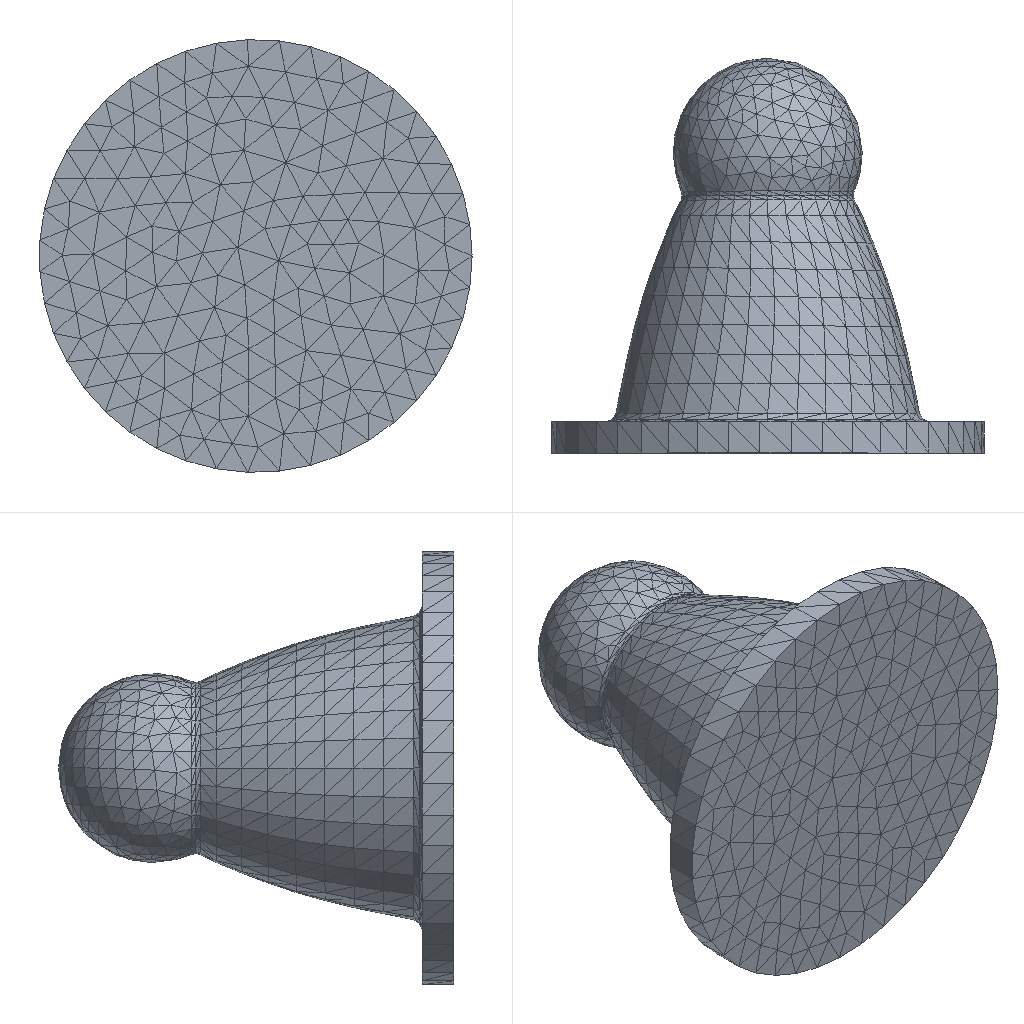Simulation study | abaqus
Set-up summary:
category,name,step,type,value,unit,region
solver,abaqus
solver,version,,,Abaqus/Standard 3DEXPERIENCE R2017x
units,not stated in the deck,,not stated
analysis,deck,,static,static
load_step,Step-1,Step-1,static
load_step,requested,,,1
mesh,nodes,,,22669
mesh,elements,,,15589
element_type,C3D10,,solid,15589
load,load commands in deck,,count,1
bc,support commands in deck,,count,7
material,Q235,,in results
check,setup vs results,,match,"per instance, exact: element labels, types and connectivity; labels of the nodes the elements use; coordinates of those nodes at SINGLE_PRECISION in 1 of 1 instance(s)"
Abaqus input file, long lists of numbers shortened:
*Heading
** Job name: Job-1 Model name: Model-1
** Generated by: Abaqus/CAE 2017
*Preprint, echo=NO, model=NO, history=NO, contact=NO
**
** PARTS
**
*Part, name=merge
*Node
      1,   10.997,          75.,           0.
      2,   14.973,   73.032,           0.
** (22667 more lines like these left out)
*Element, type=C3D10
   1,  661, 1608,  660, 1609, 3084, 3083, 3082, 3086, 3085, 3087
   2, 1610, 1611,  511, 1612, 3090, 3089, 3088, 3092, 3091, 3093
** (15587 more lines like these left out)
*Nset, nset=Set-4, generate
     1,  22669,      1
*Elset, elset=Set-4, generate
     1,  15589,      1
** Section: Section-1
*Solid Section, elset=Set-4, material=Q235
,
*End Part
**
**
** ASSEMBLY
**
*Assembly, name=Assembly
**
*Instance, name=merge-1, part=merge
*End Instance
**
*Node
      1,          10.,         143.,           0.
*Nset, nset=Set-6
 1,
*Nset, nset=Set-7, instance=merge-1
     1,     2,     3,     4,     5,     6,     7,    10,    11,    16,    17,    18,    19,    20,    21,    22
    23,    24,    25,    26,    27,    28,    29,    30,    31,    32,    33,    34,    35,    36,    37,    38
** (857 more lines like these left out)
*Elset, elset=Set-7, instance=merge-1
     1,     2,     3,     4,     5,     6,     7,     8,     9,    10,    11,    12,    13,    14,    15,    16
    17,    18,    19,    20,    21,    22,    23,    24,    25,    26,    27,    28,    29,    30,    31,    32
** (584 more lines like these left out)
*Nset, nset=Set-9, instance=merge-1
    10,    11,   234,   235,   236,   237,   238,   239,   240,   241,   242,   243,   244,   245,   246,   247
   248,   249,   250,   251,   252,   253,   254,   255,   256,   257,   258,   259,   260,   261,   262,   263
** (58 more lines like these left out)
*Elset, elset=Set-9, instance=merge-1
  5457,  5469,  5504,  5558,  5591,  5606,  5615,  5619,  5636,  5644,  5650,  5721,  5763,  5803,  5865,  5892
  5915,  5968,  6049,  6054,  6064,  6113,  6126,  6134,  6154,  6241,  6251,  6254,  6317,  6323,  6345,  6435
** (26 more lines like these left out)
*Nset, nset=Set-10, instance=merge-1
     9,   191,   192,   193,   194,   195,   196,   197,   198,   199,   200,   201,   202,   203,   204,   205
   206,   207,   208,   209,   210,   211,   212,   213,   214,   215,   216,   217,   218,   219,   220,   221
** (44 more lines like these left out)
*Elset, elset=Set-10, instance=merge-1
 3412, 3416, 3429, 3442, 3446, 3464, 3474, 3489, 3491, 3499, 3506, 3529, 3530, 3535, 3540, 3546
 3553, 3558, 3562, 3571, 3584, 3606, 3608, 3618, 3624, 3630, 3634, 3643, 3646, 3647, 3655, 3677
** (20 more lines like these left out)
*Nset, nset=Set-11
 1,
*Nset, nset=Set-12, instance=merge-1
    1,    2,    3,    4,    5,    6,   16,   17,   18,   19,   20,   21,   22,   23,   24,   25
   26,   27,   28,   29,   30,   31,   32,   33,   34,   35,   36,   37,   38,   39,   40,   41
** (347 more lines like these left out)
*Elset, elset=Set-12, instance=merge-1, generate
    1,  3403,     1
*Nset, nset=Set-13, instance=merge-1
    1,    2,    3,    4,    5,    6,   16,   17,   18,   19,   20,   21,   22,   23,   24,   25
   26,   27,   28,   29,   30,   31,   32,   33,   34,   35,   36,   37,   38,   39,   40,   41
** (347 more lines like these left out)
*Elset, elset=Set-13, instance=merge-1, generate
    1,  3403,     1
*Nset, nset=m_Set-5
 1,
*Nset, nset=p_Set-7, instance=merge-1
     1,     2,     3,     4,     5,     6,     7,    10,    11,    16,    17,    18,    19,    20,    21,    22
    23,    24,    25,    26,    27,    28,    29,    30,    31,    32,    33,    34,    35,    36,    37,    38
** (857 more lines like these left out)
*Elset, elset=p_Set-7, instance=merge-1
     1,     2,     3,     4,     5,     6,     7,     8,     9,    10,    11,    12,    13,    14,    15,    16
    17,    18,    19,    20,    21,    22,    23,    24,    25,    26,    27,    28,    29,    30,    31,    32
** (584 more lines like these left out)
*Nset, nset=p_Set-8, instance=merge-1
     1,     2,     3,     4,     5,     6,     7,    10,    11,    16,    17,    18,    19,    20,    21,    22
    23,    24,    25,    26,    27,    28,    29,    30,    31,    32,    33,    34,    35,    36,    37,    38
** (857 more lines like these left out)
*Elset, elset=p_Set-8, instance=merge-1
     1,     2,     3,     4,     5,     6,     7,     8,     9,    10,    11,    12,    13,    14,    15,    16
    17,    18,    19,    20,    21,    22,    23,    24,    25,    26,    27,    28,    29,    30,    31,    32
** (584 more lines like these left out)
*Nset, nset=p_Set-12, instance=merge-1
    1,    2,    3,    4,    5,    6,   16,   17,   18,   19,   20,   21,   22,   23,   24,   25
   26,   27,   28,   29,   30,   31,   32,   33,   34,   35,   36,   37,   38,   39,   40,   41
** (347 more lines like these left out)
*Elset, elset=p_Set-12, instance=merge-1, generate
    1,  3403,     1
*Nset, nset=p_Set-14, instance=merge-1
    1,    2,    3,    4,    5,    6,   16,   17,   18,   19,   20,   21,   22,   23,   24,   25
   26,   27,   28,   29,   30,   31,   32,   33,   34,   35,   36,   37,   38,   39,   40,   41
** (347 more lines like these left out)
*Elset, elset=p_Set-14, instance=merge-1, generate
    1,  3403,     1
*Nset, nset=p_Set-15, instance=merge-1
    1,    2,    3,    4,    5,    6,   16,   17,   18,   19,   20,   21,   22,   23,   24,   25
   26,   27,   28,   29,   30,   31,   32,   33,   34,   35,   36,   37,   38,   39,   40,   41
** (347 more lines like these left out)
*Elset, elset=p_Set-15, instance=merge-1, generate
    1,  3403,     1
*Elset, elset=_s_Surf-1_S3, internal, instance=merge-1
 11302, 11332, 11553, 11665, 11694, 11741, 11787, 11806, 11838, 11956, 12179, 12391, 12410, 12517, 12559, 12754
 12828, 12857, 12860, 12875, 12876, 12880, 12894, 12895, 12913, 12916, 12919, 12941, 12945, 12951, 12961, 12966
** (27 more lines like these left out)
*Elset, elset=_s_Surf-1_S4, internal, instance=merge-1
 12264, 12528, 13649, 13897, 14285, 14557, 14624
*Elset, elset=_s_Surf-1_S2, internal, instance=merge-1
 12865, 13239, 15133, 15136
*Elset, elset=_s_Surf-1_S1, internal, instance=merge-1
 12869, 13222, 13907, 13985, 14693, 15096
*Surface, type=ELEMENT, name=s_Surf-1
_s_Surf-1_S3, S3
_s_Surf-1_S4, S4
_s_Surf-1_S2, S2
_s_Surf-1_S1, S1
*Elset, elset=_s_Surf-2_S3, internal, instance=merge-1
 11302, 11332, 11553, 11665, 11694, 11741, 11787, 11806, 11838, 11956, 12179, 12391, 12410, 12517, 12559, 12754
 12828, 12857, 12860, 12875, 12876, 12880, 12894, 12895, 12913, 12916, 12919, 12941, 12945, 12951, 12961, 12966
** (27 more lines like these left out)
*Elset, elset=_s_Surf-2_S4, internal, instance=merge-1
 12264, 12528, 13649, 13897, 14285, 14557, 14624
*Elset, elset=_s_Surf-2_S2, internal, instance=merge-1
 12865, 13239, 15133, 15136
*Elset, elset=_s_Surf-2_S1, internal, instance=merge-1
 12869, 13222, 13907, 13985, 14693, 15096
*Surface, type=ELEMENT, name=s_Surf-2
_s_Surf-2_S3, S3
_s_Surf-2_S4, S4
_s_Surf-2_S2, S2
_s_Surf-2_S1, S1
** Constraint: Constraint-1
*Coupling, constraint name=Constraint-1, ref node=m_Set-5, surface=s_Surf-2
*Kinematic
*End Assembly
*Amplitude, name=Amp-1
             0.,              0.,              1.,             0.1,              2.,              0.,              3.,            -0.2
             4.,              0.,              5.,             0.3,              6.,              0.,              7.,            -0.4
             8.,              0.,              9.,             0.5,             10.,              0.
**
** MATERIALS
**
*Material, name=Q235
*Elastic
210000., 0.3
*Plastic
235.,0.
**
** BOUNDARY CONDITIONS
**
** Name: BC-1 Type: 对称/反对称/完全固定
*Boundary
Set-10, ENCASTRE
** ----------------------------------------------------------------
**
** STEP: Step-1
**
*Step, name=Step-1, nlgeom=YES, inc=1000
*Static, stabilize=0.0002, allsdtol=0.05, continue=NO
0.01, 10., 0.0001, 10.
**
** BOUNDARY CONDITIONS
**
** Name: BC-2 Type: 位移/转角
*Boundary, amplitude=Amp-1
Set-11, 1, 1, 1.
Set-11, 2, 2
Set-11, 3, 3
Set-11, 4, 4
Set-11, 5, 5
Set-11, 6, 6
**
** OUTPUT REQUESTS
**
*Restart, write, frequency=0
**
** FIELD OUTPUT: F-Output-1
**
*Output, field
*Node Output
CF, RF, U, V
*Element Output, directions=YES
E, LE, MISES, PE, PEEQ, PEMAG, S
*Contact Output
CDISP, CSTRESS
**
** HISTORY OUTPUT: H-Output-1
**
*Output, history, variable=PRESELECT
*End Step
Results summary:
result,step,,completed,increments=68 time=10.0/10.0
result,analysis,,,static
result,last_loadstep,,,1
result,primary field,,,U
result,reaction total,,FX,-2534.99,model units
result,reaction total,,FY,-4.032,model units
result,reaction total,,FZ,-3.155,model units